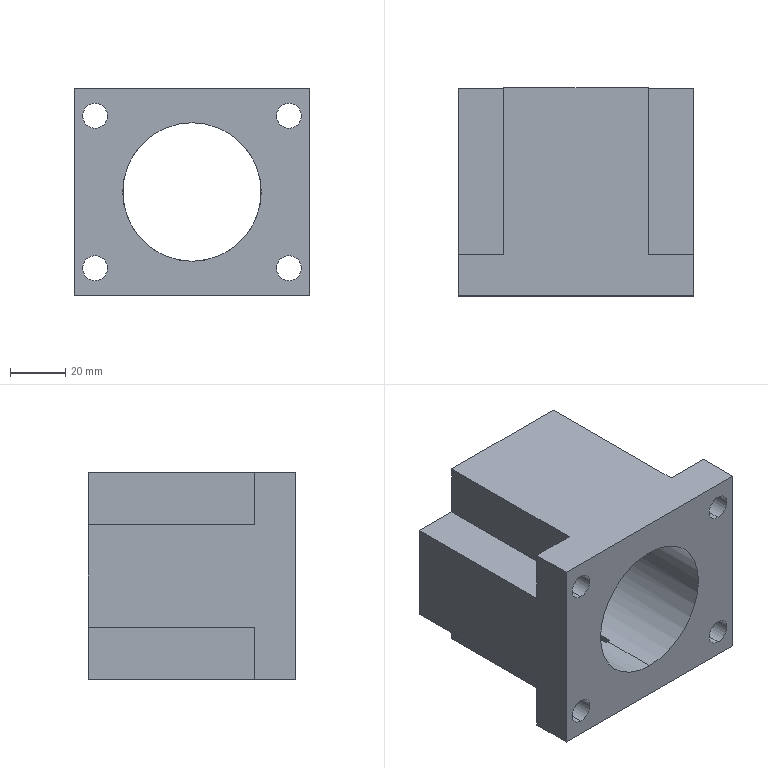Part | STEP file | 1 solid | 31 faces | box 85 x 75 x 75 mm | volume 250465 mm3 | plane 21 | cylinder 10 | commonest cylinder face diameters 9 x8 50 x2